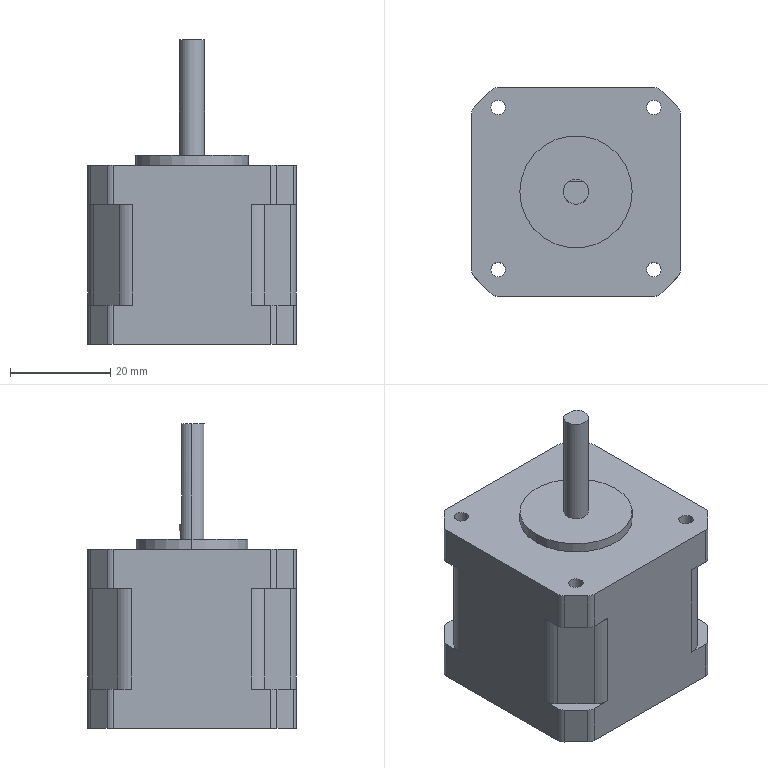Part | SolidWorks | features ICE 2, MBimport 1 | 1 solid | 66 faces | box 41.6 x 41.6 x 60.7 mm | volume 59288 mm3 | cylinder 36 | plane 30 | commonest cylinder face diameters 3.6 x16 2.9 x8 7.6 x8 5 x2 22.4 x2